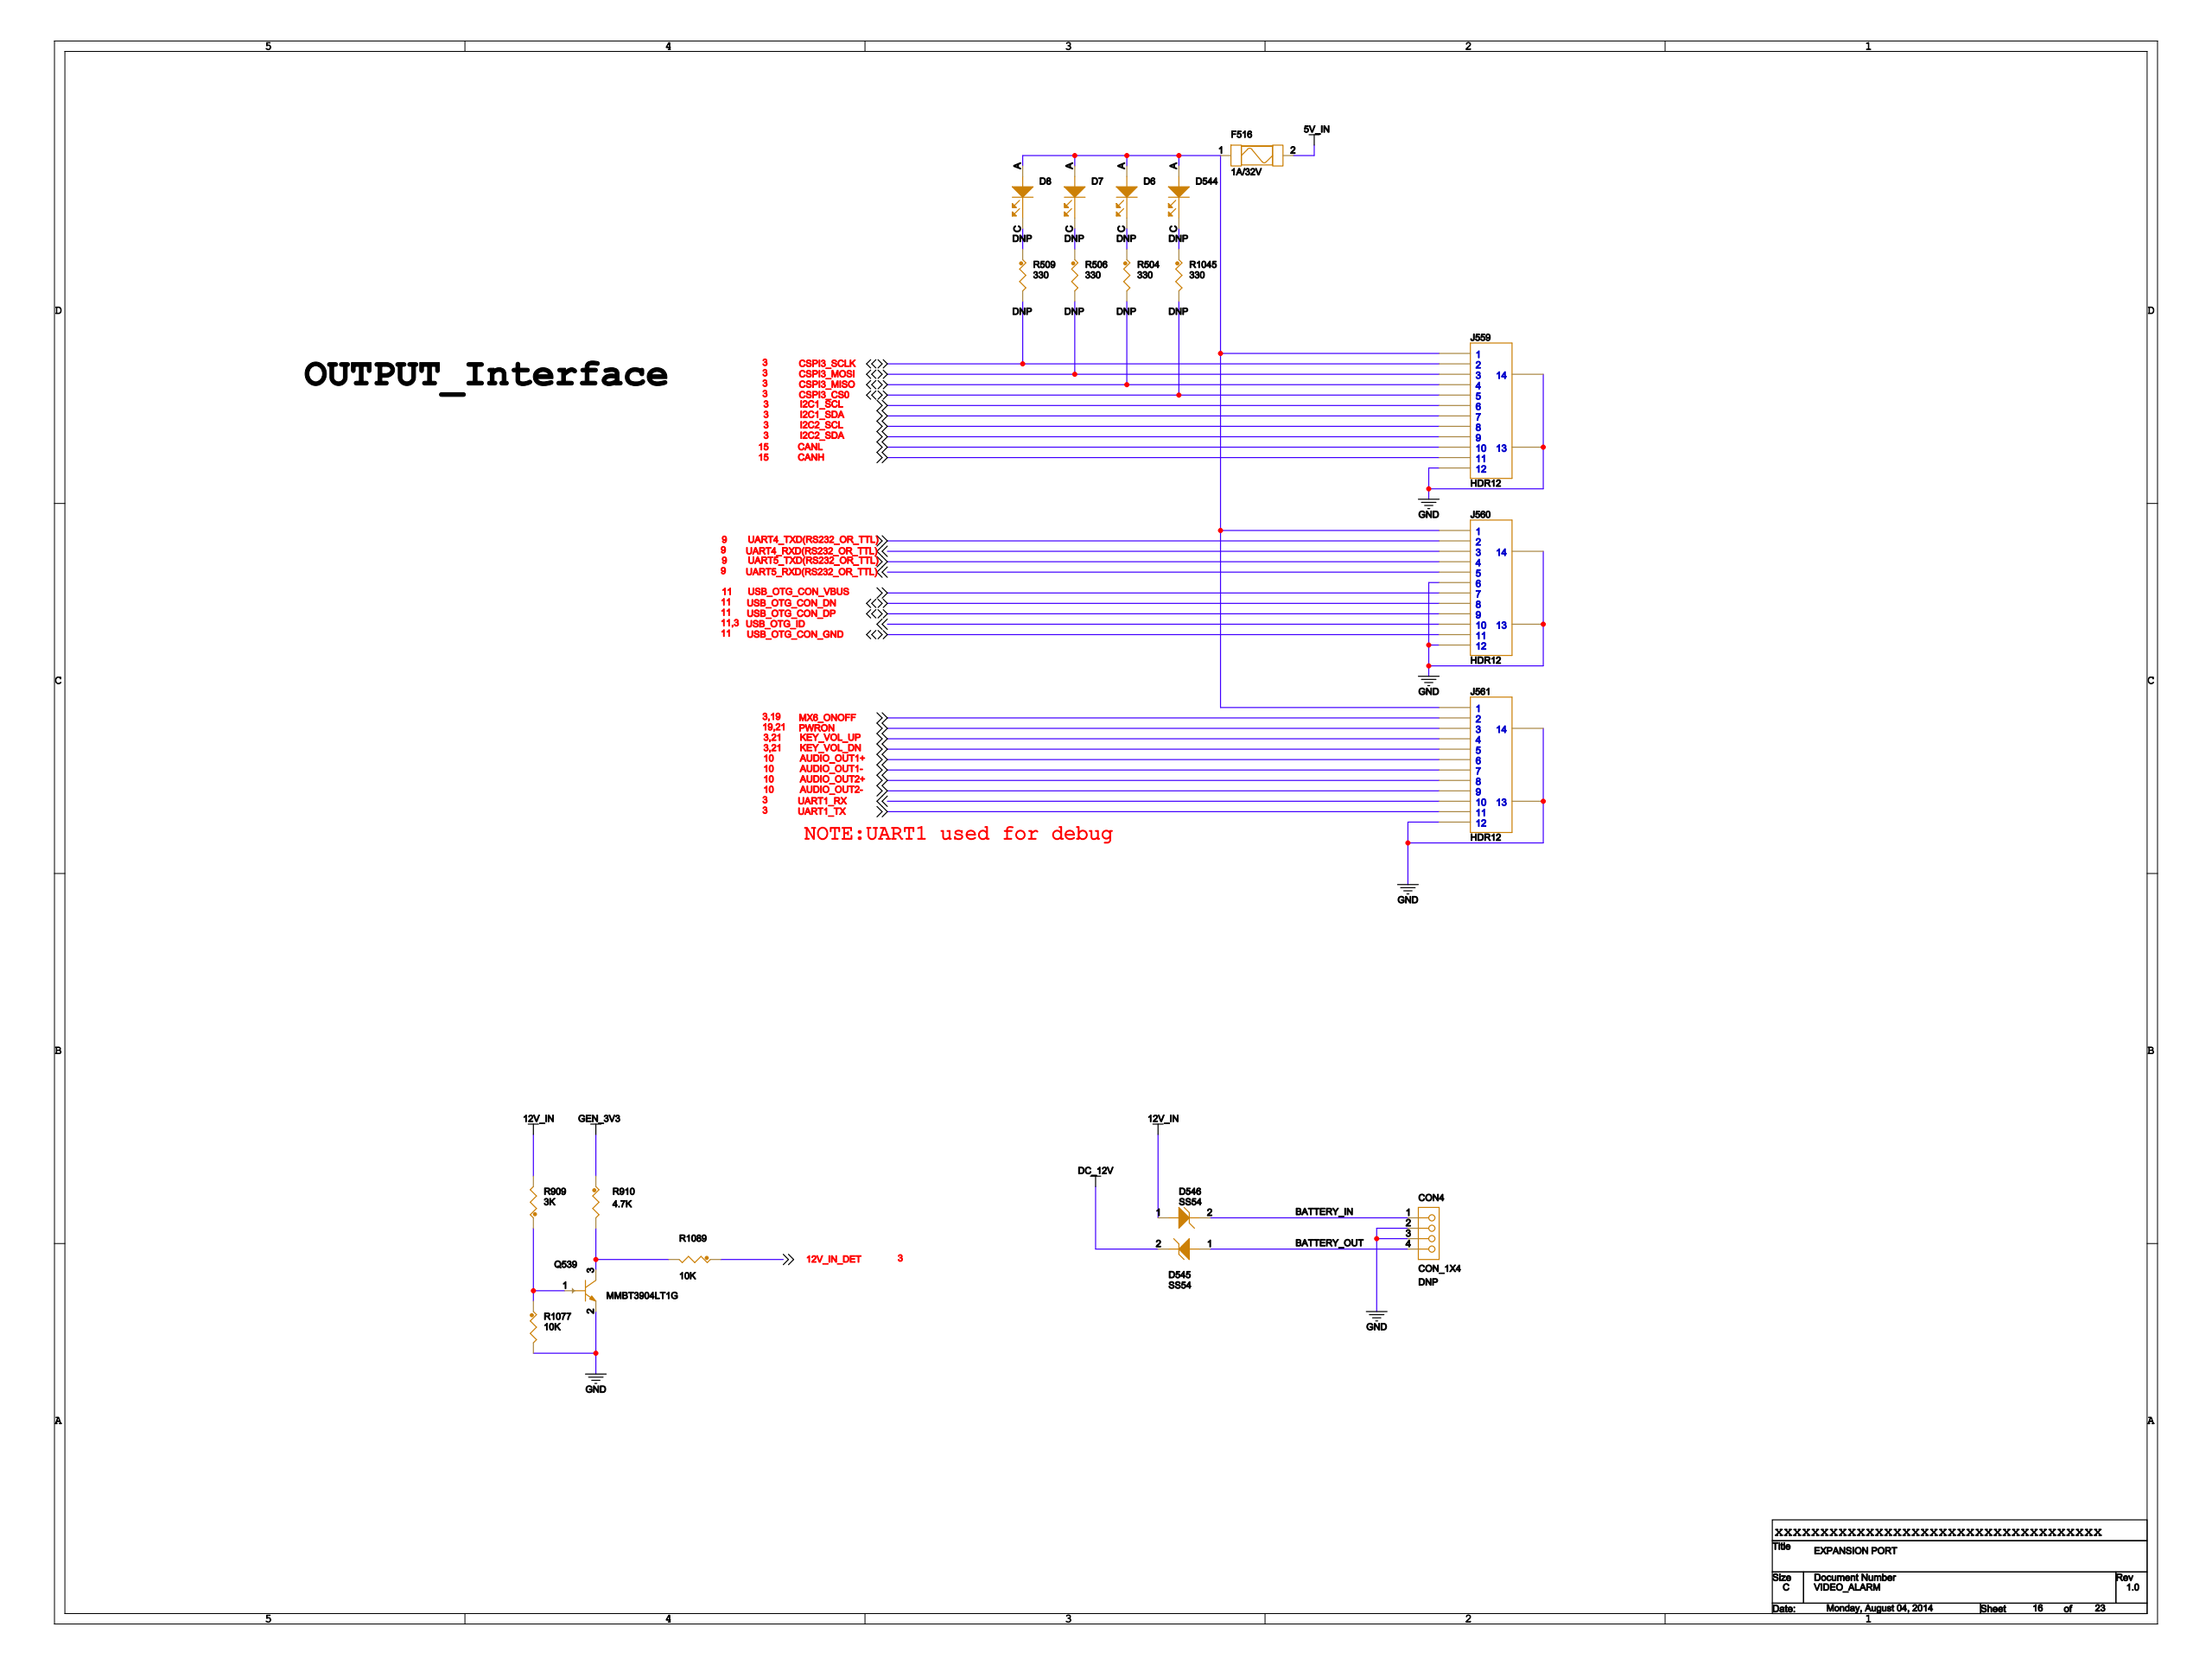Circuit board | Cadence Allegro | 994 parts | 728 nets | one sheet of the schematic
Parts on this sheet (reference | value | footprint):
CON4 | CON_1X4 | CON_TB_4F_2P5_9X10P5
D544 | LED_GREEN | LED_0603
D545 | SS54 | DO-214AB
D546 | SS54 | DO-214AB
F516 | 1A/32V | 1206_CC
J559 | HDR12 | HDR12
J560 | HDR12 | HDR12
J561 | HDR12 | HDR12
Q539 | MMBT3904LT1G | SOT23
R504 | 330 | 0603_CC
R506 | 330 | 0603_CC
R509 | 330 | 0603_CC
R909 | 3K | 0603_CC
R910 | 4.7K | 0603_CC
R1045 | 330 | 0603_CC
R1077 | 10K | 0603_CC
R1089 | 10K | 0603_CC
Nets of these parts (net: part-pin ...):
GND: CON4-2 CON4-3 J559-12 J559-13 J559-14 J560-6 J560-12 J560-13 J560-14 J561-12 J561-13 J561-14 Q539-2 R1077-2
12V_IN: D546-1 R909-2
PWRON: J561-3
GEN_3V3: R910-1
UART4_RXD: J560-3
UART5_TXD: J560-4
UART4_TXD: J560-2
UART5_RXD: J560-5
DC_12V: D545-2
5V_IN: F516-2
N16905417: D544-A F516-1 J559-1 J560-1 J561-1
MX6_ONOFF: J561-2
KEY_VOL_UP: J561-4
KEY_VOL_DN: J561-5
AUDIO_OUT1-: J561-7
AUDIO_OUT1+: J561-6
AUDIO_OUT2+: J561-8
UART1_RX: J561-10
AUDIO_OUT2-: J561-9
UART1_TX: J561-11
USB_OTG_CON_VBUS: J560-7
USB_OTG_CON_DN: J560-8
USB_OTG_ID: J560-10
USB_OTG_CON_DP: J560-9
USB_OTG_CON_GND: J560-11
CSPI3_SCLK: J559-2 R509-2
CSPI3_MISO: J559-4 R504-2
CSPI3_MOSI: J559-3 R506-2
CSPI3_CS0: J559-5 R1045-2
I2C1_SDA: J559-7
I2C1_SCL: J559-6
I2C2_SCL: J559-8
CANL: J559-10
I2C2_SDA: J559-9
CANH: J559-11
N16905414: R509-1
N16910084: R506-1
N16910087: R504-1
N22612022: D544-C R1045-1
BATTERY_IN: CON4-1 D546-2
BATTERY_OUT: CON4-4 D545-1
12V_IN_DET: R1089-1
N22811044: Q539-3 R910-2 R1089-2
N22811057: Q539-1 R909-1 R1077-1